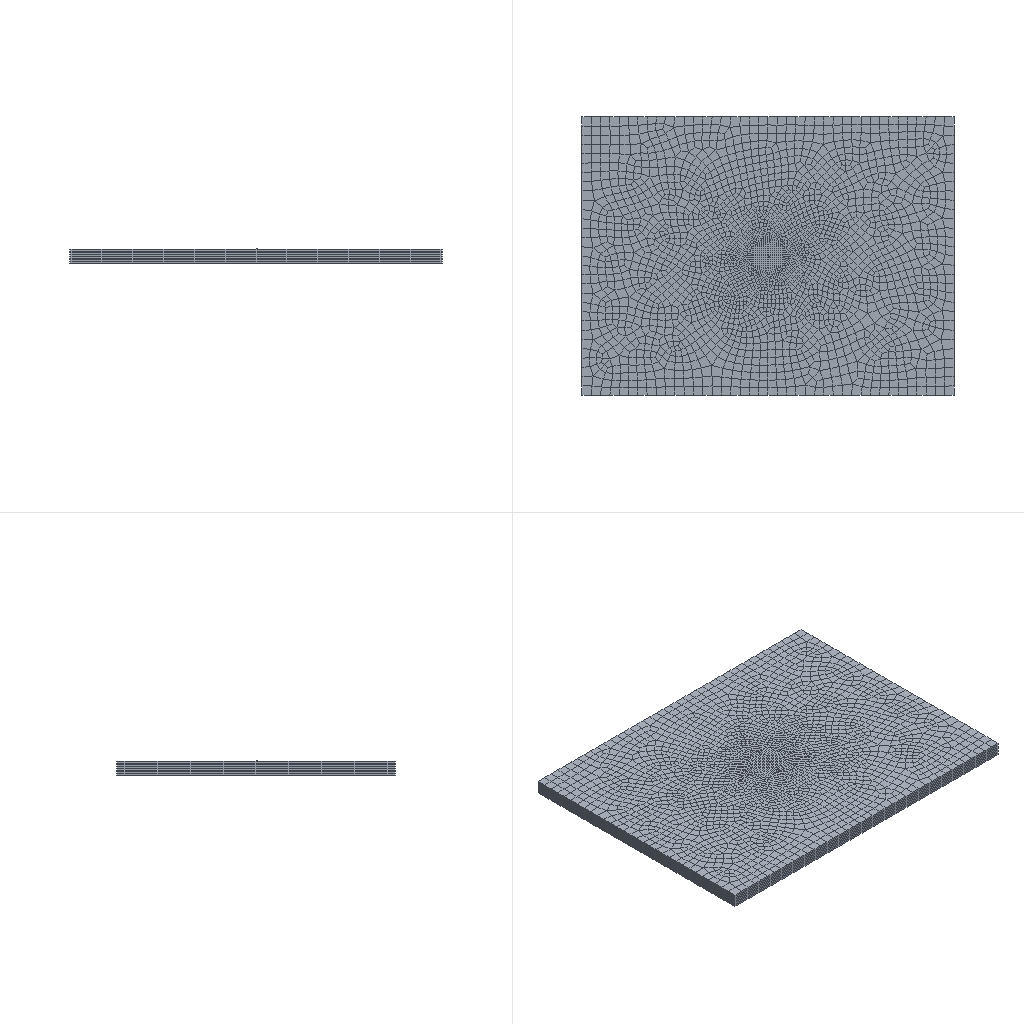Simulation study | abaqus
Set-up summary:
category,name,step,type,value,unit,region
solver,abaqus,,Abaqus/CAE 2024
units,SI m-kg-s (Pa),,inferred,E=7e+10 density=2600
analysis,Step-1,,dynamic explicit,nlgeom=True; time_period=0.003
mesh,nodes,,,30287
mesh,elements,,,26224
element_type,C3D8R,,,26224
material,nisha,,E,7e+10
material,nisha,,nu,0.23
material,nisha,,density,2600
material,shuilunji,,E,2e+11
material,shuilunji,,nu,0.33
material,shuilunji,,density,7900
material,shuilunji,,yield,5.4e+08
material,shuilunji,,behaviors,plastic
section,shuilunji,,solid section,,,Set-3
section,nisha,,solid section,,,Set-1
load,Predefined,initial,initial condition velocity
bc,BC-1,initial,encastre,[dofs=ENCASTRE],,Set-1
bc,BC-2,initial,velocity,"[dofs=rx,ry,rz,x,y n=5]",,_PickedSet26
contact,Int-2,initial,general contact,interaction=IntProp-1; friction=0; behavior=hard
constraint,rigid body,,,1
Abaqus input file, long lists of numbers shortened:
*Heading
** Job name: deck Model name: Model-1
** Generated by: Abaqus/CAE 2024
*Preprint, echo=NO, model=NO, history=NO, contact=NO
**
** PARTS
**
*Part, name=diban
*Node
      1, -0.01625, -0.00875,           0.
      2, -0.01625, 0.01125,           0.
** (27655 more lines like these left out)
*Element, type=C3D8R
   1,  116,  885, 7477,  689,    1,   17,  437,   62
   2,  885,  886, 7478, 7477,   17,   18,  438,  437
** (24014 more lines like these left out)
*Nset, nset=Set-3, generate
     1,  27657,      1
*Elset, elset=Set-3, generate
     1,  24016,      1
** Section: diban
*Solid Section, elset=Set-3, material=shuilunji
,
*End Part
**
*Part, name=nisha
*Node
      1,           0.,           0.,           0.
      2,           0.,           0., 0.0005
** (2627 more lines like these left out)
*Element, type=C3D8R
  1,  232,  233, 1270, 1225,    8,    9,  167,  166
  2,  233,  234, 1271, 1270,    9,   10,  168,  167
** (2206 more lines like these left out)
*Nset, nset=Set-1, generate
    1,  2629,     1
*Elset, elset=Set-1, generate
    1,  2208,     1
** Section: nisha
*Solid Section, elset=Set-1, material=nisha
,
*End Part
**
**
** ASSEMBLY
**
*Assembly, name=Assembly
**
*Instance, name=diban-1, part=diban
*End Instance
**
*Instance, name=nisha-1, part=nisha
          0.,           0.,       0.0155
*End Instance
**
*Node
      1,           0.,           0., 0.0155
*Nset, nset=Set-1, instance=diban-1
    1,    2,    3,    4,    9,   10,   11,   12,   17,   18,   19,   20,   21,   22,   23,   24
   25,   26,   27,   28,   29,   30,   31,   32,   33,   34,   35,   36,   37,   38,   39,   40
** (183 more lines like these left out)
*Elset, elset=Set-1, instance=diban-1, generate
 1201,  4052,     1
*Nset, nset=b_Set-2, instance=nisha-1, generate
    1,  2629,     1
*Elset, elset=b_Set-2, instance=nisha-1, generate
    1,  2208,     1
*Nset, nset=s_Set-5, instance=diban-1
    5,    6,    7,    8,   13,   14,   15,   16,   63,   64,   65,   66,   67,   68,   69,   70
   71,   72,   73,   74,   75,   76,   77,   78,   79,   80,   81,   82,   83,   84,   85,   86
** (183 more lines like these left out)
*Elset, elset=s_Set-5, instance=diban-1, generate
 21165,  24016,      1
*Nset, nset=_PickedSet25, internal
 1,
*Nset, nset=_PickedSet26, internal
 1,
*Nset, nset=_PickedSet27, internal
 1,
*Elset, elset=_m_Surf-1_S2, internal, instance=diban-1, generate
 21165,  24016,      1
*Elset, elset=_m_Surf-1_S1, internal, instance=diban-1, generate
 1051,  1200,     1
*Surface, type=ELEMENT, name=m_Surf-1
_m_Surf-1_S2, S2
_m_Surf-1_S1, S1
*Elset, elset=_m_Surf-2_S4, internal, instance=nisha-1
  181,  182,  183,  184,  185,  186,  187,  188,  189,  190,  191,  192,  193,  194,  195,  196
  197,  198,  199,  200,  201,  202,  203,  204,  205,  206,  207,  208,  209,  210,  247,  248
** (18 more lines like these left out)
*Elset, elset=_m_Surf-2_S3, internal, instance=nisha-1
  211,  212,  213,  214,  215,  216,  217,  218,  219,  220,  221,  222,  223,  224,  225,  226
  227,  228,  229,  230,  231,  232,  233,  234,  235,  236,  237,  238,  239,  240,  241,  242
** (15 more lines like these left out)
*Elset, elset=_m_Surf-2_S2, internal, instance=nisha-1
  553,  554,  555,  556,  557,  558,  559,  560,  561,  562,  563,  564,  565,  566,  567,  568
  569,  570,  571,  572,  573,  574,  575,  576,  577,  578,  579,  580,  581,  582,  583,  584
** (10 more lines like these left out)
*Surface, type=ELEMENT, name=m_Surf-2
_m_Surf-2_S4, S4
_m_Surf-2_S3, S3
_m_Surf-2_S2, S2
*Elset, elset=_s_Surf-2_S2, internal, instance=diban-1, generate
 21165,  24016,      1
*Elset, elset=_s_Surf-2_S1, internal, instance=diban-1, generate
 1051,  1200,     1
*Surface, type=ELEMENT, name=s_Surf-2
_s_Surf-2_S2, S2
_s_Surf-2_S1, S1
** Constraint: Constraint-1
*Rigid Body, ref node=_PickedSet25, elset=b_Set-2
*End Assembly
**
** MATERIALS
**
*Material, name=nisha
*Density
2600.,
*Elastic
 7e+10, 0.23
*Material, name=shuilunji
*Density
7900.,
*Elastic
 2e+11, 0.33
*Plastic
     5.4e+08,   0.
     6.5e+08, 0.01
 6.95563e+08, 0.02
 7.30526e+08, 0.03
     7.6e+08, 0.04
 7.85967e+08, 0.05
 8.09444e+08, 0.06
 8.31033e+08, 0.07
**
** INTERACTION PROPERTIES
**
*Surface Interaction, name=IntProp-1
*Friction
0.,
*Surface Behavior, pressure-overclosure=HARD
**
** BOUNDARY CONDITIONS
**
** Name: BC-1 Type: Symmetry/Antisymmetry/Encastre
*Boundary
Set-1, ENCASTRE
** Name: BC-2 Type: Velocity/Angular velocity
*Boundary, type=VELOCITY
_PickedSet26, 1, 1
_PickedSet26, 2, 2
_PickedSet26, 4, 4
_PickedSet26, 5, 5
_PickedSet26, 6, 6
**
** PREDEFINED FIELDS
**
** Name: Predefined Field-1   Type: Velocity
*Initial Conditions, type=VELOCITY
_PickedSet27, 3, -15.6
**
** INTERACTIONS
**
** Interaction: Int-2
*Contact, op=NEW
*Contact Inclusions, ALL EXTERIOR
*Contact Property Assignment
 ,  , IntProp-1
** ----------------------------------------------------------------
**
** STEP: Step-1
**
*Step, name=Step-1, nlgeom=YES
*Dynamic, Explicit
, 0.003
*Bulk Viscosity
0.06, 1.2
** Mass Scaling: Semi-Automatic
**               Whole Model
*Fixed Mass Scaling, factor=10000.
**
** OUTPUT REQUESTS
**
*Restart, write, number interval=1, time marks=NO
**
** FIELD OUTPUT: F-Output-1
**
*Output, field, variable=PRESELECT
**
** HISTORY OUTPUT: H-Output-1
**
*Output, history, variable=PRESELECT, frequency=1
*End Step
Results summary:
result,odb.job_status,,,JOB_STATUS_COMPLETED_SUCCESSFULLY,"consistent, unstated (Abaqus has no unit system)"
result,steps[0].procedure,Step-1,,"*DYNAMIC, EXPLICIT","consistent, unstated (Abaqus has no unit system)"
result,steps[0].time_period,Step-1,,0.003,"consistent, unstated (Abaqus has no unit system)"
result,steps[0].n_frames,Step-1,,21,"consistent, unstated (Abaqus has no unit system)"
result,steps[0].last_frame.id,Step-1,,120,"consistent, unstated (Abaqus has no unit system)"
result,steps[0].last_frame.value,Step-1,,0.003,"consistent, unstated (Abaqus has no unit system)"
result,steps[0].last_frame.description,Step-1,,Increment       120: Step Time =   3.0000E-03,"consistent, unstated (Abaqus has no unit system)"
result,steps[0].completed,Step-1,,True,"consistent, unstated (Abaqus has no unit system)"
result,steps[0].max_U_magnitude,Step-1,,0.0333,"consistent, unstated (Abaqus has no unit system)"
result,steps[0].max_S_mises,Step-1,,4.46599e+07,"consistent, unstated (Abaqus has no unit system)"
result,steps[0].RF_sum[1],Step-1,,176.763,"consistent, unstated (Abaqus has no unit system)"
result,steps[0].RF_sum[2],Step-1,,-5.515,"consistent, unstated (Abaqus has no unit system)"
result,steps[0].RF_sum[3],Step-1,,-221.45,"consistent, unstated (Abaqus has no unit system)"
result,steps[0].diagnostic.n_increments,Step-1,,21,"consistent, unstated (Abaqus has no unit system)"